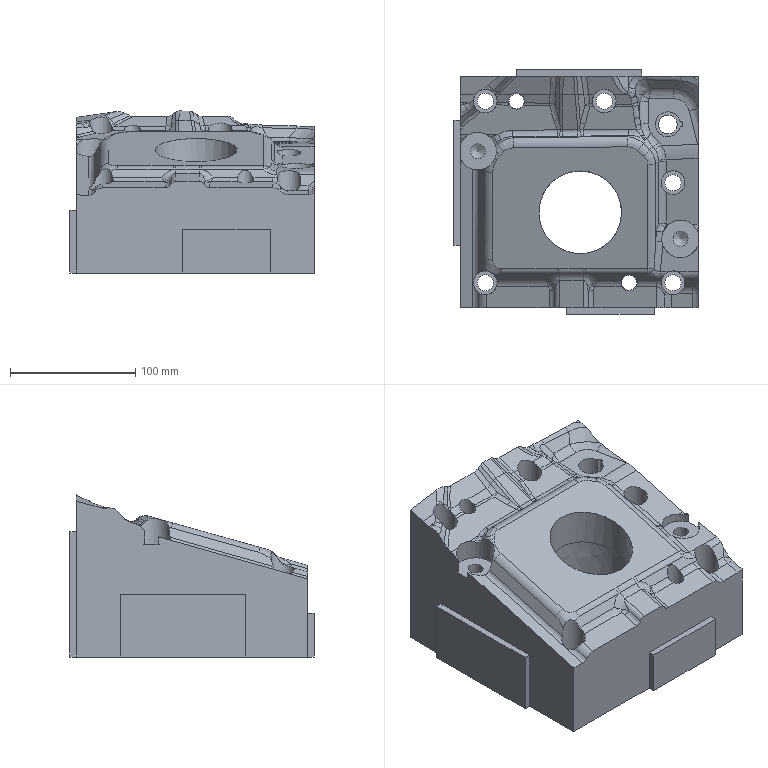Part | NX | features solid 2 | 1 solid | 227 faces | box 195 x 195 x 129.396 mm | volume 2924081 mm3 | spline 88 | cylinder 80 | plane 56 | cone 2 | sphere 1 | commonest cylinder face diameters 16 x19 10 x15 20 x10 13 x7 19 x5 12 x4